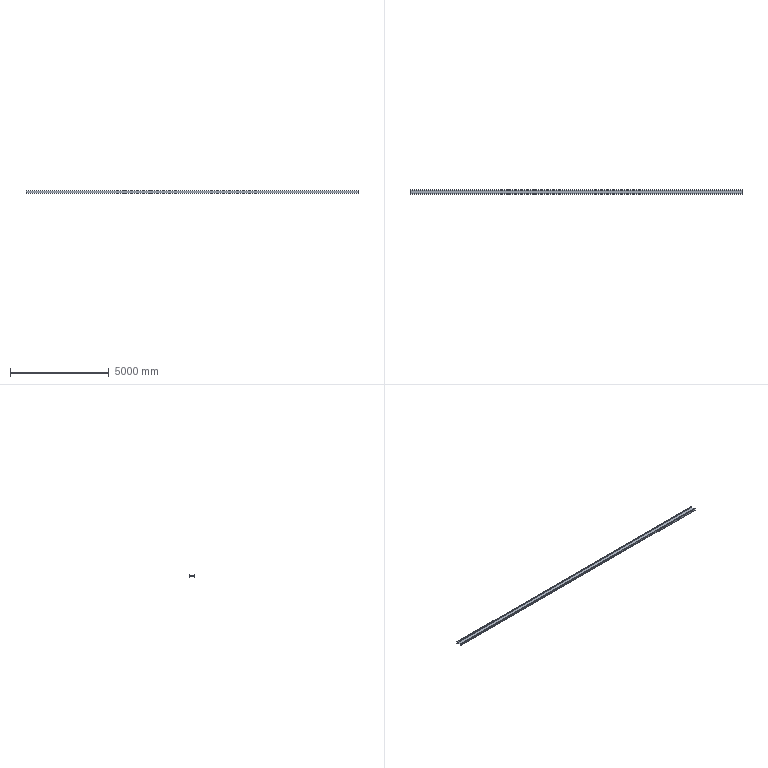Part | SolidWorks | features Fillet 2, Extrusion 1 | 1 solid | 22 faces | box 16840 x 250 x 118 mm | volume 87084540 mm3 | plane 14 | cylinder 8 | commonest cylinder face diameters 10 x4 20 x4
STEP:
#1=CARTESIAN_POINT('',(16840.,3.431,59.));
#2=VERTEX_POINT('',#1);
#3=CARTESIAN_POINT('',(16840.,0.,59.));
#4=VERTEX_POINT('',#3);
#5=CARTESIAN_POINT('',(16840.,7.667,59.));
#6=DIRECTION('',(0.,-1.,0.));
#7=VECTOR('',#6,1000.);
#8=LINE('',#5,#7);
#9=EDGE_CURVE('',#2,#4,#8,.T.);
#10=ORIENTED_EDGE('',*,*,#9,.F.);
#11=CARTESIAN_POINT('',(0.,3.431,59.));
#12=VERTEX_POINT('',#11);
#13=CARTESIAN_POINT('',(16840.,3.431,59.));
#14=DIRECTION('',(-1.,0.,0.));
#15=VECTOR('',#14,1000.);
#16=LINE('',#13,#15);
#17=EDGE_CURVE('',#2,#12,#16,.T.);
#18=ORIENTED_EDGE('',*,*,#17,.T.);
#19=CARTESIAN_POINT('',(0.,0.,59.));
#20=VERTEX_POINT('',#19);
#21=CARTESIAN_POINT('',(0.,7.667,59.));
#22=DIRECTION('',(0.,-1.,0.));
#23=VECTOR('',#22,1000.);
#24=LINE('',#21,#23);
#25=EDGE_CURVE('',#12,#20,#24,.T.);
#26=ORIENTED_EDGE('',*,*,#25,.T.);
#27=CARTESIAN_POINT('',(16840.,0.,59.));
#28=DIRECTION('',(-1.,0.,0.));
#29=VECTOR('',#28,1000.);
#30=LINE('',#27,#29);
#31=EDGE_CURVE('',#4,#20,#30,.T.);
#32=ORIENTED_EDGE('',*,*,#31,.F.);
#33=EDGE_LOOP('',(#10,#18,#26,#32));
#34=FACE_OUTER_BOUND('',#33,.T.);
#35=CARTESIAN_POINT('',(16840.,7.667,59.));
#36=DIRECTION('',(0.,0.,-1.));
#37=DIRECTION('',(-1.,0.,0.));
#38=AXIS2_PLACEMENT_3D('',#35,#36,#37);
#39=PLANE('',#38);
#40=ADVANCED_FACE('',(#34),#39,.F.);
#41=CARTESIAN_POINT('',(0.,0.,-59.));
#42=VERTEX_POINT('',#41);
#43=CARTESIAN_POINT('',(0.,0.,59.));
#44=DIRECTION('',(0.,0.,-1.));
#45=VECTOR('',#44,1000.);
#46=LINE('',#43,#45);
#47=EDGE_CURVE('',#20,#42,#46,.T.);
#48=ORIENTED_EDGE('',*,*,#47,.T.);
#49=CARTESIAN_POINT('',(16840.,0.,-59.));
#50=VERTEX_POINT('',#49);
#51=CARTESIAN_POINT('',(16840.,0.,-59.));
#52=DIRECTION('',(-1.,0.,0.));
#53=VECTOR('',#52,1000.);
#54=LINE('',#51,#53);
#55=EDGE_CURVE('',#50,#42,#54,.T.);
#56=ORIENTED_EDGE('',*,*,#55,.F.);
#57=CARTESIAN_POINT('',(16840.,0.,59.));
#58=DIRECTION('',(0.,0.,-1.));
#59=VECTOR('',#58,1000.);
#60=LINE('',#57,#59);
#61=EDGE_CURVE('',#4,#50,#60,.T.);
#62=ORIENTED_EDGE('',*,*,#61,.F.);
#63=ORIENTED_EDGE('',*,*,#31,.T.);
#64=EDGE_LOOP('',(#48,#56,#62,#63));
#65=FACE_OUTER_BOUND('',#64,.T.);
#66=CARTESIAN_POINT('',(16840.,0.,59.));
#67=DIRECTION('',(0.,1.,0.));
#68=DIRECTION('',(0.,0.,1.));
#69=AXIS2_PLACEMENT_3D('',#66,#67,#68);
#70=PLANE('',#69);
#71=ADVANCED_FACE('',(#65),#70,.F.);
#72=CARTESIAN_POINT('',(0.,3.431,-59.));
#73=VERTEX_POINT('',#72);
#74=CARTESIAN_POINT('',(0.,7.667,-59.));
#75=DIRECTION('',(0.,1.,0.));
#76=VECTOR('',#75,1000.);
#77=LINE('',#74,#76);
#78=EDGE_CURVE('',#42,#73,#77,.T.);
#79=ORIENTED_EDGE('',*,*,#78,.T.);
#80=CARTESIAN_POINT('',(16840.,3.431,-59.));
#81=VERTEX_POINT('',#80);
#82=CARTESIAN_POINT('',(16840.,3.431,-59.));
#83=DIRECTION('',(1.,0.,0.));
#84=VECTOR('',#83,1000.);
#85=LINE('',#82,#84);
#86=EDGE_CURVE('',#73,#81,#85,.T.);
#87=ORIENTED_EDGE('',*,*,#86,.T.);
#88=CARTESIAN_POINT('',(16840.,7.667,-59.));
#89=DIRECTION('',(0.,1.,0.));
#90=VECTOR('',#89,1000.);
#91=LINE('',#88,#90);
#92=EDGE_CURVE('',#50,#81,#91,.T.);
#93=ORIENTED_EDGE('',*,*,#92,.F.);
#94=ORIENTED_EDGE('',*,*,#55,.T.);
#95=EDGE_LOOP('',(#79,#87,#93,#94));
#96=FACE_OUTER_BOUND('',#95,.T.);
#97=CARTESIAN_POINT('',(16840.,7.667,-59.));
#98=DIRECTION('',(0.,0.,1.));
#99=DIRECTION('',(1.,0.,0.));
#100=AXIS2_PLACEMENT_3D('',#97,#98,#99);
#101=PLANE('',#100);
#102=ADVANCED_FACE('',(#96),#101,.F.);
#103=CARTESIAN_POINT('',(16840.,8.363,-54.822));
#104=VERTEX_POINT('',#103);
#105=CARTESIAN_POINT('',(16840.,15.274,-13.356));
#106=VERTEX_POINT('',#105);
#107=CARTESIAN_POINT('',(16840.,16.667,-5.));
#108=DIRECTION('',(0.,0.1644,0.9864));
#109=VECTOR('',#108,1000.);
#110=LINE('',#107,#109);
#111=EDGE_CURVE('',#104,#106,#110,.T.);
#112=ORIENTED_EDGE('',*,*,#111,.F.);
#113=CARTESIAN_POINT('',(0.,8.363,-54.822));
#114=VERTEX_POINT('',#113);
#115=CARTESIAN_POINT('',(16840.,8.363,-54.822));
#116=DIRECTION('',(-1.,0.,0.));
#117=VECTOR('',#116,1000.);
#118=LINE('',#115,#117);
#119=EDGE_CURVE('',#104,#114,#118,.T.);
#120=ORIENTED_EDGE('',*,*,#119,.T.);
#121=CARTESIAN_POINT('',(0.,15.274,-13.356));
#122=VERTEX_POINT('',#121);
#123=CARTESIAN_POINT('',(0.,16.667,-5.));
#124=DIRECTION('',(0.,0.1644,0.9864));
#125=VECTOR('',#124,1000.);
#126=LINE('',#123,#125);
#127=EDGE_CURVE('',#114,#122,#126,.T.);
#128=ORIENTED_EDGE('',*,*,#127,.T.);
#129=CARTESIAN_POINT('',(16840.,15.274,-13.356));
#130=DIRECTION('',(1.,0.,0.));
#131=VECTOR('',#130,1000.);
#132=LINE('',#129,#131);
#133=EDGE_CURVE('',#122,#106,#132,.T.);
#134=ORIENTED_EDGE('',*,*,#133,.T.);
#135=EDGE_LOOP('',(#112,#120,#128,#134));
#136=FACE_OUTER_BOUND('',#135,.T.);
#137=CARTESIAN_POINT('',(16840.,16.667,-5.));
#138=DIRECTION('',(0.,-0.9864,0.1644));
#139=DIRECTION('',(0.,-0.1644,-0.9864));
#140=AXIS2_PLACEMENT_3D('',#137,#138,#139);
#141=PLANE('',#140);
#142=ADVANCED_FACE('',(#136),#141,.F.);
#143=CARTESIAN_POINT('',(0.,25.138,-5.));
#144=VERTEX_POINT('',#143);
#145=CARTESIAN_POINT('',(0.,224.862,-5.));
#146=VERTEX_POINT('',#145);
#147=CARTESIAN_POINT('',(0.,233.333,-5.));
#148=DIRECTION('',(0.,1.,0.));
#149=VECTOR('',#148,1000.);
#150=LINE('',#147,#149);
#151=EDGE_CURVE('',#144,#146,#150,.T.);
#152=ORIENTED_EDGE('',*,*,#151,.T.);
#153=CARTESIAN_POINT('',(16840.,224.862,-5.));
#154=VERTEX_POINT('',#153);
#155=CARTESIAN_POINT('',(16840.,224.862,-5.));
#156=DIRECTION('',(1.,0.,0.));
#157=VECTOR('',#156,1000.);
#158=LINE('',#155,#157);
#159=EDGE_CURVE('',#146,#154,#158,.T.);
#160=ORIENTED_EDGE('',*,*,#159,.T.);
#161=CARTESIAN_POINT('',(16840.,25.138,-5.));
#162=VERTEX_POINT('',#161);
#163=CARTESIAN_POINT('',(16840.,233.333,-5.));
#164=DIRECTION('',(0.,1.,0.));
#165=VECTOR('',#164,1000.);
#166=LINE('',#163,#165);
#167=EDGE_CURVE('',#162,#154,#166,.T.);
#168=ORIENTED_EDGE('',*,*,#167,.F.);
#169=CARTESIAN_POINT('',(0.,25.138,-5.));
#170=DIRECTION('',(-1.,0.,0.));
#171=VECTOR('',#170,1000.);
#172=LINE('',#169,#171);
#173=EDGE_CURVE('',#162,#144,#172,.T.);
#174=ORIENTED_EDGE('',*,*,#173,.T.);
#175=EDGE_LOOP('',(#152,#160,#168,#174));
#176=FACE_OUTER_BOUND('',#175,.T.);
#177=CARTESIAN_POINT('',(16840.,233.333,-5.));
#178=DIRECTION('',(0.,0.,1.));
#179=DIRECTION('',(0.,-1.,0.));
#180=AXIS2_PLACEMENT_3D('',#177,#178,#179);
#181=PLANE('',#180);
#182=ADVANCED_FACE('',(#176),#181,.F.);
#183=CARTESIAN_POINT('',(0.,234.726,-13.356));
#184=VERTEX_POINT('',#183);
#185=CARTESIAN_POINT('',(0.,241.637,-54.822));
#186=VERTEX_POINT('',#185);
#187=CARTESIAN_POINT('',(0.,242.333,-59.));
#188=DIRECTION('',(0.,0.1644,-0.9864));
#189=VECTOR('',#188,1000.);
#190=LINE('',#187,#189);
#191=EDGE_CURVE('',#184,#186,#190,.T.);
#192=ORIENTED_EDGE('',*,*,#191,.T.);
#193=CARTESIAN_POINT('',(16840.,241.637,-54.822));
#194=VERTEX_POINT('',#193);
#195=CARTESIAN_POINT('',(16840.,241.637,-54.822));
#196=DIRECTION('',(1.,0.,0.));
#197=VECTOR('',#196,1000.);
#198=LINE('',#195,#197);
#199=EDGE_CURVE('',#186,#194,#198,.T.);
#200=ORIENTED_EDGE('',*,*,#199,.T.);
#201=CARTESIAN_POINT('',(16840.,234.726,-13.356));
#202=VERTEX_POINT('',#201);
#203=CARTESIAN_POINT('',(16840.,242.333,-59.));
#204=DIRECTION('',(0.,0.1644,-0.9864));
#205=VECTOR('',#204,1000.);
#206=LINE('',#203,#205);
#207=EDGE_CURVE('',#202,#194,#206,.T.);
#208=ORIENTED_EDGE('',*,*,#207,.F.);
#209=CARTESIAN_POINT('',(0.,234.726,-13.356));
#210=DIRECTION('',(-1.,0.,0.));
#211=VECTOR('',#210,1000.);
#212=LINE('',#209,#211);
#213=EDGE_CURVE('',#202,#184,#212,.T.);
#214=ORIENTED_EDGE('',*,*,#213,.T.);
#215=EDGE_LOOP('',(#192,#200,#208,#214));
#216=FACE_OUTER_BOUND('',#215,.T.);
#217=CARTESIAN_POINT('',(16840.,242.333,-59.));
#218=DIRECTION('',(0.,0.9864,0.1644));
#219=DIRECTION('',(0.,-0.1644,0.9864));
#220=AXIS2_PLACEMENT_3D('',#217,#218,#219);
#221=PLANE('',#220);
#222=ADVANCED_FACE('',(#216),#221,.F.);
#223=CARTESIAN_POINT('',(16840.,246.569,-59.));
#224=VERTEX_POINT('',#223);
#225=CARTESIAN_POINT('',(16840.,250.,-59.));
#226=VERTEX_POINT('',#225);
#227=CARTESIAN_POINT('',(16840.,250.,-59.));
#228=DIRECTION('',(0.,1.,0.));
#229=VECTOR('',#228,1000.);
#230=LINE('',#227,#229);
#231=EDGE_CURVE('',#224,#226,#230,.T.);
#232=ORIENTED_EDGE('',*,*,#231,.F.);
#233=CARTESIAN_POINT('',(0.,246.569,-59.));
#234=VERTEX_POINT('',#233);
#235=CARTESIAN_POINT('',(16840.,246.569,-59.));
#236=DIRECTION('',(-1.,0.,0.));
#237=VECTOR('',#236,1000.);
#238=LINE('',#235,#237);
#239=EDGE_CURVE('',#224,#234,#238,.T.);
#240=ORIENTED_EDGE('',*,*,#239,.T.);
#241=CARTESIAN_POINT('',(0.,250.,-59.));
#242=VERTEX_POINT('',#241);
#243=CARTESIAN_POINT('',(0.,250.,-59.));
#244=DIRECTION('',(0.,1.,0.));
#245=VECTOR('',#244,1000.);
#246=LINE('',#243,#245);
#247=EDGE_CURVE('',#234,#242,#246,.T.);
#248=ORIENTED_EDGE('',*,*,#247,.T.);
#249=CARTESIAN_POINT('',(16840.,250.,-59.));
#250=DIRECTION('',(-1.,0.,0.));
#251=VECTOR('',#250,1000.);
#252=LINE('',#249,#251);
#253=EDGE_CURVE('',#226,#242,#252,.T.);
#254=ORIENTED_EDGE('',*,*,#253,.F.);
#255=EDGE_LOOP('',(#232,#240,#248,#254));
#256=FACE_OUTER_BOUND('',#255,.T.);
#257=CARTESIAN_POINT('',(16840.,250.,-59.));
#258=DIRECTION('',(0.,0.,1.));
#259=DIRECTION('',(0.,-1.,0.));
#260=AXIS2_PLACEMENT_3D('',#257,#258,#259);
#261=PLANE('',#260);
#262=ADVANCED_FACE('',(#256),#261,.F.);
#263=CARTESIAN_POINT('',(0.,250.,59.));
#264=VERTEX_POINT('',#263);
#265=CARTESIAN_POINT('',(0.,250.,59.));
#266=DIRECTION('',(0.,0.,1.));
#267=VECTOR('',#266,1000.);
#268=LINE('',#265,#267);
#269=EDGE_CURVE('',#242,#264,#268,.T.);
#270=ORIENTED_EDGE('',*,*,#269,.T.);
#271=CARTESIAN_POINT('',(16840.,250.,59.));
#272=VERTEX_POINT('',#271);
#273=CARTESIAN_POINT('',(16840.,250.,59.));
#274=DIRECTION('',(-1.,0.,0.));
#275=VECTOR('',#274,1000.);
#276=LINE('',#273,#275);
#277=EDGE_CURVE('',#272,#264,#276,.T.);
#278=ORIENTED_EDGE('',*,*,#277,.F.);
#279=CARTESIAN_POINT('',(16840.,250.,59.));
#280=DIRECTION('',(0.,0.,1.));
#281=VECTOR('',#280,1000.);
#282=LINE('',#279,#281);
#283=EDGE_CURVE('',#226,#272,#282,.T.);
#284=ORIENTED_EDGE('',*,*,#283,.F.);
#285=ORIENTED_EDGE('',*,*,#253,.T.);
#286=EDGE_LOOP('',(#270,#278,#284,#285));
#287=FACE_OUTER_BOUND('',#286,.T.);
#288=CARTESIAN_POINT('',(16840.,250.,59.));
#289=DIRECTION('',(0.,-1.,0.));
#290=DIRECTION('',(0.,0.,-1.));
#291=AXIS2_PLACEMENT_3D('',#288,#289,#290);
#292=PLANE('',#291);
#293=ADVANCED_FACE('',(#287),#292,.F.);
#294=CARTESIAN_POINT('',(0.,246.569,59.));
#295=VERTEX_POINT('',#294);
#296=CARTESIAN_POINT('',(0.,250.,59.));
#297=DIRECTION('',(0.,-1.,0.));
#298=VECTOR('',#297,1000.);
#299=LINE('',#296,#298);
#300=EDGE_CURVE('',#264,#295,#299,.T.);
#301=ORIENTED_EDGE('',*,*,#300,.T.);
#302=CARTESIAN_POINT('',(16840.,246.569,59.));
#303=VERTEX_POINT('',#302);
#304=CARTESIAN_POINT('',(16840.,246.569,59.));
#305=DIRECTION('',(1.,0.,0.));
#306=VECTOR('',#305,1000.);
#307=LINE('',#304,#306);
#308=EDGE_CURVE('',#295,#303,#307,.T.);
#309=ORIENTED_EDGE('',*,*,#308,.T.);
#310=CARTESIAN_POINT('',(16840.,250.,59.));
#311=DIRECTION('',(0.,-1.,0.));
#312=VECTOR('',#311,1000.);
#313=LINE('',#310,#312);
#314=EDGE_CURVE('',#272,#303,#313,.T.);
#315=ORIENTED_EDGE('',*,*,#314,.F.);
#316=ORIENTED_EDGE('',*,*,#277,.T.);
#317=EDGE_LOOP('',(#301,#309,#315,#316));
#318=FACE_OUTER_BOUND('',#317,.T.);
#319=CARTESIAN_POINT('',(16840.,250.,59.));
#320=DIRECTION('',(0.,0.,-1.));
#321=DIRECTION('',(-1.,0.,0.));
#322=AXIS2_PLACEMENT_3D('',#319,#320,#321);
#323=PLANE('',#322);
#324=ADVANCED_FACE('',(#318),#323,.F.);
#325=CARTESIAN_POINT('',(16840.,241.637,54.822));
#326=VERTEX_POINT('',#325);
#327=CARTESIAN_POINT('',(16840.,234.726,13.356));
#328=VERTEX_POINT('',#327);
#329=CARTESIAN_POINT('',(16840.,242.333,59.));
#330=DIRECTION('',(0.,-0.1644,-0.9864));
#331=VECTOR('',#330,1000.);
#332=LINE('',#329,#331);
#333=EDGE_CURVE('',#326,#328,#332,.T.);
#334=ORIENTED_EDGE('',*,*,#333,.F.);
#335=CARTESIAN_POINT('',(0.,241.637,54.822));
#336=VERTEX_POINT('',#335);
#337=CARTESIAN_POINT('',(16840.,241.637,54.822));
#338=DIRECTION('',(-1.,0.,0.));
#339=VECTOR('',#338,1000.);
#340=LINE('',#337,#339);
#341=EDGE_CURVE('',#326,#336,#340,.T.);
#342=ORIENTED_EDGE('',*,*,#341,.T.);
#343=CARTESIAN_POINT('',(0.,234.726,13.356));
#344=VERTEX_POINT('',#343);
#345=CARTESIAN_POINT('',(0.,242.333,59.));
#346=DIRECTION('',(0.,-0.1644,-0.9864));
#347=VECTOR('',#346,1000.);
#348=LINE('',#345,#347);
#349=EDGE_CURVE('',#336,#344,#348,.T.);
#350=ORIENTED_EDGE('',*,*,#349,.T.);
#351=CARTESIAN_POINT('',(16840.,234.726,13.356));
#352=DIRECTION('',(1.,0.,0.));
#353=VECTOR('',#352,1000.);
#354=LINE('',#351,#353);
#355=EDGE_CURVE('',#344,#328,#354,.T.);
#356=ORIENTED_EDGE('',*,*,#355,.T.);
#357=EDGE_LOOP('',(#334,#342,#350,#356));
#358=FACE_OUTER_BOUND('',#357,.T.);
#359=CARTESIAN_POINT('',(16840.,242.333,59.));
#360=DIRECTION('',(0.,0.9864,-0.1644));
#361=DIRECTION('',(0.,0.1644,0.9864));
#362=AXIS2_PLACEMENT_3D('',#359,#360,#361);
#363=PLANE('',#362);
#364=ADVANCED_FACE('',(#358),#363,.F.);
#365=CARTESIAN_POINT('',(0.,224.862,5.));
#366=VERTEX_POINT('',#365);
#367=CARTESIAN_POINT('',(0.,25.138,5.));
#368=VERTEX_POINT('',#367);
#369=CARTESIAN_POINT('',(0.,233.333,5.));
#370=DIRECTION('',(0.,-1.,0.));
#371=VECTOR('',#370,1000.);
#372=LINE('',#369,#371);
#373=EDGE_CURVE('',#366,#368,#372,.T.);
#374=ORIENTED_EDGE('',*,*,#373,.T.);
#375=CARTESIAN_POINT('',(16840.,25.138,5.));
#376=VERTEX_POINT('',#375);
#377=CARTESIAN_POINT('',(16840.,25.138,5.));
#378=DIRECTION('',(1.,0.,0.));
#379=VECTOR('',#378,1000.);
#380=LINE('',#377,#379);
#381=EDGE_CURVE('',#368,#376,#380,.T.);
#382=ORIENTED_EDGE('',*,*,#381,.T.);
#383=CARTESIAN_POINT('',(16840.,224.862,5.));
#384=VERTEX_POINT('',#383);
#385=CARTESIAN_POINT('',(16840.,233.333,5.));
#386=DIRECTION('',(0.,-1.,0.));
#387=VECTOR('',#386,1000.);
#388=LINE('',#385,#387);
#389=EDGE_CURVE('',#384,#376,#388,.T.);
#390=ORIENTED_EDGE('',*,*,#389,.F.);
#391=CARTESIAN_POINT('',(0.,224.862,5.));
#392=DIRECTION('',(-1.,0.,0.));
#393=VECTOR('',#392,1000.);
#394=LINE('',#391,#393);
#395=EDGE_CURVE('',#384,#366,#394,.T.);
#396=ORIENTED_EDGE('',*,*,#395,.T.);
#397=EDGE_LOOP('',(#374,#382,#390,#396));
#398=FACE_OUTER_BOUND('',#397,.T.);
#399=CARTESIAN_POINT('',(16840.,233.333,5.));
#400=DIRECTION('',(0.,0.,-1.));
#401=DIRECTION('',(0.,1.,0.));
#402=AXIS2_PLACEMENT_3D('',#399,#400,#401);
#403=PLANE('',#402);
#404=ADVANCED_FACE('',(#398),#403,.F.);
#405=CARTESIAN_POINT('',(0.,15.274,13.356));
#406=VERTEX_POINT('',#405);
#407=CARTESIAN_POINT('',(0.,8.363,54.822));
#408=VERTEX_POINT('',#407);
#409=CARTESIAN_POINT('',(0.,16.667,5.));
#410=DIRECTION('',(0.,-0.1644,0.9864));
#411=VECTOR('',#410,1000.);
#412=LINE('',#409,#411);
#413=EDGE_CURVE('',#406,#408,#412,.T.);
#414=ORIENTED_EDGE('',*,*,#413,.T.);
#415=CARTESIAN_POINT('',(16840.,8.363,54.822));
#416=VERTEX_POINT('',#415);
#417=CARTESIAN_POINT('',(16840.,8.363,54.822));
#418=DIRECTION('',(1.,0.,0.));
#419=VECTOR('',#418,1000.);
#420=LINE('',#417,#419);
#421=EDGE_CURVE('',#408,#416,#420,.T.);
#422=ORIENTED_EDGE('',*,*,#421,.T.);
#423=CARTESIAN_POINT('',(16840.,15.274,13.356));
#424=VERTEX_POINT('',#423);
#425=CARTESIAN_POINT('',(16840.,16.667,5.));
#426=DIRECTION('',(0.,-0.1644,0.9864));
#427=VECTOR('',#426,1000.);
#428=LINE('',#425,#427);
#429=EDGE_CURVE('',#424,#416,#428,.T.);
#430=ORIENTED_EDGE('',*,*,#429,.F.);
#431=CARTESIAN_POINT('',(0.,15.274,13.356));
#432=DIRECTION('',(-1.,0.,0.));
#433=VECTOR('',#432,1000.);
#434=LINE('',#431,#433);
#435=EDGE_CURVE('',#424,#406,#434,.T.);
#436=ORIENTED_EDGE('',*,*,#435,.T.);
#437=EDGE_LOOP('',(#414,#422,#430,#436));
#438=FACE_OUTER_BOUND('',#437,.T.);
#439=CARTESIAN_POINT('',(16840.,16.667,5.));
#440=DIRECTION('',(0.,-0.9864,-0.1644));
#441=DIRECTION('',(0.,0.1644,-0.9864));
#442=AXIS2_PLACEMENT_3D('',#439,#440,#441);
#443=PLANE('',#442);
#444=ADVANCED_FACE('',(#438),#443,.F.);
#445=ORIENTED_EDGE('',*,*,#314,.T.);
#446=CARTESIAN_POINT('',(16840.,246.569,54.));
#447=DIRECTION('',(1.,0.,0.));
#448=DIRECTION('',(0.,0.,-1.));
#449=AXIS2_PLACEMENT_3D('',#446,#447,#448);
#450=CIRCLE('',#449,5.);
#451=EDGE_CURVE('',#303,#326,#450,.T.);
#452=ORIENTED_EDGE('',*,*,#451,.T.);
#453=ORIENTED_EDGE('',*,*,#333,.T.);
#454=CARTESIAN_POINT('',(16840.,224.862,15.));
#455=DIRECTION('',(-1.,0.,0.));
#456=DIRECTION('',(0.,0.,-1.));
#457=AXIS2_PLACEMENT_3D('',#454,#455,#456);
#458=CIRCLE('',#457,10.);
#459=EDGE_CURVE('',#328,#384,#458,.T.);
#460=ORIENTED_EDGE('',*,*,#459,.T.);
#461=ORIENTED_EDGE('',*,*,#389,.T.);
#462=CARTESIAN_POINT('',(16840.,25.138,15.));
#463=DIRECTION('',(-1.,0.,0.));
#464=DIRECTION('',(0.,0.,-1.));
#465=AXIS2_PLACEMENT_3D('',#462,#463,#464);
#466=CIRCLE('',#465,10.);
#467=EDGE_CURVE('',#376,#424,#466,.T.);
#468=ORIENTED_EDGE('',*,*,#467,.T.);
#469=ORIENTED_EDGE('',*,*,#429,.T.);
#470=CARTESIAN_POINT('',(16840.,3.431,54.));
#471=DIRECTION('',(1.,0.,0.));
#472=DIRECTION('',(0.,0.,-1.));
#473=AXIS2_PLACEMENT_3D('',#470,#471,#472);
#474=CIRCLE('',#473,5.);
#475=EDGE_CURVE('',#416,#2,#474,.T.);
#476=ORIENTED_EDGE('',*,*,#475,.T.);
#477=ORIENTED_EDGE('',*,*,#9,.T.);
#478=ORIENTED_EDGE('',*,*,#61,.T.);
#479=ORIENTED_EDGE('',*,*,#92,.T.);
#480=CARTESIAN_POINT('',(16840.,3.431,-54.));
#481=DIRECTION('',(1.,0.,0.));
#482=DIRECTION('',(0.,0.,-1.));
#483=AXIS2_PLACEMENT_3D('',#480,#481,#482);
#484=CIRCLE('',#483,5.);
#485=EDGE_CURVE('',#81,#104,#484,.T.);
#486=ORIENTED_EDGE('',*,*,#485,.T.);
#487=ORIENTED_EDGE('',*,*,#111,.T.);
#488=CARTESIAN_POINT('',(16840.,25.138,-15.));
#489=DIRECTION('',(-1.,0.,0.));
#490=DIRECTION('',(0.,0.,-1.));
#491=AXIS2_PLACEMENT_3D('',#488,#489,#490);
#492=CIRCLE('',#491,10.);
#493=EDGE_CURVE('',#106,#162,#492,.T.);
#494=ORIENTED_EDGE('',*,*,#493,.T.);
#495=ORIENTED_EDGE('',*,*,#167,.T.);
#496=CARTESIAN_POINT('',(16840.,224.862,-15.));
#497=DIRECTION('',(-1.,0.,0.));
#498=DIRECTION('',(0.,0.,-1.));
#499=AXIS2_PLACEMENT_3D('',#496,#497,#498);
#500=CIRCLE('',#499,10.);
#501=EDGE_CURVE('',#154,#202,#500,.T.);
#502=ORIENTED_EDGE('',*,*,#501,.T.);
#503=ORIENTED_EDGE('',*,*,#207,.T.);
#504=CARTESIAN_POINT('',(16840.,246.569,-54.));
#505=DIRECTION('',(1.,0.,0.));
#506=DIRECTION('',(0.,0.,-1.));
#507=AXIS2_PLACEMENT_3D('',#504,#505,#506);
#508=CIRCLE('',#507,5.);
#509=EDGE_CURVE('',#194,#224,#508,.T.);
#510=ORIENTED_EDGE('',*,*,#509,.T.);
#511=ORIENTED_EDGE('',*,*,#231,.T.);
#512=ORIENTED_EDGE('',*,*,#283,.T.);
#513=EDGE_LOOP('',(#445,#452,#453,#460,#461,#468,#469,#476,#477,#478,#479,#486,#487,#494,#495,#502,#503,#510,#511,#512));
#514=FACE_OUTER_BOUND('',#513,.T.);
#515=CARTESIAN_POINT('',(16840.,250.,59.));
#516=DIRECTION('',(1.,0.,0.));
#517=DIRECTION('',(0.,0.,-1.));
#518=AXIS2_PLACEMENT_3D('',#515,#516,#517);
#519=PLANE('',#518);
#520=ADVANCED_FACE('',(#514),#519,.T.);
#521=ORIENTED_EDGE('',*,*,#349,.F.);
#522=CARTESIAN_POINT('',(0.,246.569,54.));
#523=DIRECTION('',(-1.,0.,0.));
#524=DIRECTION('',(0.,0.,-1.));
#525=AXIS2_PLACEMENT_3D('',#522,#523,#524);
#526=CIRCLE('',#525,5.);
#527=EDGE_CURVE('',#336,#295,#526,.T.);
#528=ORIENTED_EDGE('',*,*,#527,.T.);
#529=ORIENTED_EDGE('',*,*,#300,.F.);
#530=ORIENTED_EDGE('',*,*,#269,.F.);
#531=ORIENTED_EDGE('',*,*,#247,.F.);
#532=CARTESIAN_POINT('',(0.,246.569,-54.));
#533=DIRECTION('',(-1.,0.,0.));
#534=DIRECTION('',(0.,0.,-1.));
#535=AXIS2_PLACEMENT_3D('',#532,#533,#534);
#536=CIRCLE('',#535,5.);
#537=EDGE_CURVE('',#234,#186,#536,.T.);
#538=ORIENTED_EDGE('',*,*,#537,.T.);
#539=ORIENTED_EDGE('',*,*,#191,.F.);
#540=CARTESIAN_POINT('',(0.,224.862,-15.));
#541=DIRECTION('',(1.,0.,0.));
#542=DIRECTION('',(0.,0.,-1.));
#543=AXIS2_PLACEMENT_3D('',#540,#541,#542);
#544=CIRCLE('',#543,10.);
#545=EDGE_CURVE('',#184,#146,#544,.T.);
#546=ORIENTED_EDGE('',*,*,#545,.T.);
#547=ORIENTED_EDGE('',*,*,#151,.F.);
#548=CARTESIAN_POINT('',(0.,25.138,-15.));
#549=DIRECTION('',(1.,0.,0.));
#550=DIRECTION('',(0.,0.,-1.));
#551=AXIS2_PLACEMENT_3D('',#548,#549,#550);
#552=CIRCLE('',#551,10.);
#553=EDGE_CURVE('',#144,#122,#552,.T.);
#554=ORIENTED_EDGE('',*,*,#553,.T.);
#555=ORIENTED_EDGE('',*,*,#127,.F.);
#556=CARTESIAN_POINT('',(0.,3.431,-54.));
#557=DIRECTION('',(-1.,0.,0.));
#558=DIRECTION('',(0.,0.,-1.));
#559=AXIS2_PLACEMENT_3D('',#556,#557,#558);
#560=CIRCLE('',#559,5.);
#561=EDGE_CURVE('',#114,#73,#560,.T.);
#562=ORIENTED_EDGE('',*,*,#561,.T.);
#563=ORIENTED_EDGE('',*,*,#78,.F.);
#564=ORIENTED_EDGE('',*,*,#47,.F.);
#565=ORIENTED_EDGE('',*,*,#25,.F.);
#566=CARTESIAN_POINT('',(0.,3.431,54.));
#567=DIRECTION('',(-1.,0.,0.));
#568=DIRECTION('',(0.,0.,-1.));
#569=AXIS2_PLACEMENT_3D('',#566,#567,#568);
#570=CIRCLE('',#569,5.);
#571=EDGE_CURVE('',#12,#408,#570,.T.);
#572=ORIENTED_EDGE('',*,*,#571,.T.);
#573=ORIENTED_EDGE('',*,*,#413,.F.);
#574=CARTESIAN_POINT('',(0.,25.138,15.));
#575=DIRECTION('',(1.,0.,0.));
#576=DIRECTION('',(0.,0.,-1.));
#577=AXIS2_PLACEMENT_3D('',#574,#575,#576);
#578=CIRCLE('',#577,10.);
#579=EDGE_CURVE('',#406,#368,#578,.T.);
#580=ORIENTED_EDGE('',*,*,#579,.T.);
#581=ORIENTED_EDGE('',*,*,#373,.F.);
#582=CARTESIAN_POINT('',(0.,224.862,15.));
#583=DIRECTION('',(1.,0.,0.));
#584=DIRECTION('',(0.,0.,-1.));
#585=AXIS2_PLACEMENT_3D('',#582,#583,#584);
#586=CIRCLE('',#585,10.);
#587=EDGE_CURVE('',#366,#344,#586,.T.);
#588=ORIENTED_EDGE('',*,*,#587,.T.);
#589=EDGE_LOOP('',(#521,#528,#529,#530,#531,#538,#539,#546,#547,#554,#555,#562,#563,#564,#565,#572,#573,#580,#581,#588));
#590=FACE_OUTER_BOUND('',#589,.T.);
#591=CARTESIAN_POINT('',(0.,250.,59.));
#592=DIRECTION('',(1.,0.,0.));
#593=DIRECTION('',(0.,0.,-1.));
#594=AXIS2_PLACEMENT_3D('',#591,#592,#593);
#595=PLANE('',#594);
#596=ADVANCED_FACE('',(#590),#595,.F.);
#597=ORIENTED_EDGE('',*,*,#501,.F.);
#598=ORIENTED_EDGE('',*,*,#159,.F.);
#599=ORIENTED_EDGE('',*,*,#545,.F.);
#600=ORIENTED_EDGE('',*,*,#213,.F.);
#601=EDGE_LOOP('',(#597,#598,#599,#600));
#602=FACE_OUTER_BOUND('',#601,.T.);
#603=CARTESIAN_POINT('',(16840.,224.862,-15.));
#604=DIRECTION('',(1.,0.,0.));
#605=DIRECTION('',(0.,0.,-1.));
#606=AXIS2_PLACEMENT_3D('',#603,#604,#605);
#607=CYLINDRICAL_SURFACE('',#606,10.);
#608=ADVANCED_FACE('',(#602),#607,.F.);
#609=ORIENTED_EDGE('',*,*,#493,.F.);
#610=ORIENTED_EDGE('',*,*,#133,.F.);
#611=ORIENTED_EDGE('',*,*,#553,.F.);
#612=ORIENTED_EDGE('',*,*,#173,.F.);
#613=EDGE_LOOP('',(#609,#610,#611,#612));
#614=FACE_OUTER_BOUND('',#613,.T.);
#615=CARTESIAN_POINT('',(16840.,25.138,-15.));
#616=DIRECTION('',(1.,0.,0.));
#617=DIRECTION('',(0.,0.,-1.));
#618=AXIS2_PLACEMENT_3D('',#615,#616,#617);
#619=CYLINDRICAL_SURFACE('',#618,10.);
#620=ADVANCED_FACE('',(#614),#619,.F.);
#621=ORIENTED_EDGE('',*,*,#467,.F.);
#622=ORIENTED_EDGE('',*,*,#381,.F.);
#623=ORIENTED_EDGE('',*,*,#579,.F.);
#624=ORIENTED_EDGE('',*,*,#435,.F.);
#625=EDGE_LOOP('',(#621,#622,#623,#624));
#626=FACE_OUTER_BOUND('',#625,.T.);
#627=CARTESIAN_POINT('',(16840.,25.138,15.));
#628=DIRECTION('',(1.,0.,0.));
#629=DIRECTION('',(0.,0.,-1.));
#630=AXIS2_PLACEMENT_3D('',#627,#628,#629);
#631=CYLINDRICAL_SURFACE('',#630,10.);
#632=ADVANCED_FACE('',(#626),#631,.F.);
#633=ORIENTED_EDGE('',*,*,#459,.F.);
#634=ORIENTED_EDGE('',*,*,#355,.F.);
#635=ORIENTED_EDGE('',*,*,#587,.F.);
#636=ORIENTED_EDGE('',*,*,#395,.F.);
#637=EDGE_LOOP('',(#633,#634,#635,#636));
#638=FACE_OUTER_BOUND('',#637,.T.);
#639=CARTESIAN_POINT('',(16840.,224.862,15.));
#640=DIRECTION('',(1.,0.,0.));
#641=DIRECTION('',(0.,0.,-1.));
#642=AXIS2_PLACEMENT_3D('',#639,#640,#641);
#643=CYLINDRICAL_SURFACE('',#642,10.);
#644=ADVANCED_FACE('',(#638),#643,.F.);
#645=ORIENTED_EDGE('',*,*,#451,.F.);
#646=ORIENTED_EDGE('',*,*,#308,.F.);
#647=ORIENTED_EDGE('',*,*,#527,.F.);
#648=ORIENTED_EDGE('',*,*,#341,.F.);
#649=EDGE_LOOP('',(#645,#646,#647,#648));
#650=FACE_OUTER_BOUND('',#649,.T.);
#651=CARTESIAN_POINT('',(16840.,246.569,54.));
#652=DIRECTION('',(-1.,0.,0.));
#653=DIRECTION('',(0.,0.,1.));
#654=AXIS2_PLACEMENT_3D('',#651,#652,#653);
#655=CYLINDRICAL_SURFACE('',#654,5.);
#656=ADVANCED_FACE('',(#650),#655,.T.);
#657=ORIENTED_EDGE('',*,*,#475,.F.);
#658=ORIENTED_EDGE('',*,*,#421,.F.);
#659=ORIENTED_EDGE('',*,*,#571,.F.);
#660=ORIENTED_EDGE('',*,*,#17,.F.);
#661=EDGE_LOOP('',(#657,#658,#659,#660));
#662=FACE_OUTER_BOUND('',#661,.T.);
#663=CARTESIAN_POINT('',(16840.,3.431,54.));
#664=DIRECTION('',(-1.,0.,0.));
#665=DIRECTION('',(0.,0.,1.));
#666=AXIS2_PLACEMENT_3D('',#663,#664,#665);
#667=CYLINDRICAL_SURFACE('',#666,5.);
#668=ADVANCED_FACE('',(#662),#667,.T.);
#669=ORIENTED_EDGE('',*,*,#485,.F.);
#670=ORIENTED_EDGE('',*,*,#86,.F.);
#671=ORIENTED_EDGE('',*,*,#561,.F.);
#672=ORIENTED_EDGE('',*,*,#119,.F.);
#673=EDGE_LOOP('',(#669,#670,#671,#672));
#674=FACE_OUTER_BOUND('',#673,.T.);
#675=CARTESIAN_POINT('',(16840.,3.431,-54.));
#676=DIRECTION('',(-1.,0.,0.));
#677=DIRECTION('',(0.,0.,1.));
#678=AXIS2_PLACEMENT_3D('',#675,#676,#677);
#679=CYLINDRICAL_SURFACE('',#678,5.);
#680=ADVANCED_FACE('',(#674),#679,.T.);
#681=ORIENTED_EDGE('',*,*,#509,.F.);
#682=ORIENTED_EDGE('',*,*,#199,.F.);
#683=ORIENTED_EDGE('',*,*,#537,.F.);
#684=ORIENTED_EDGE('',*,*,#239,.F.);
#685=EDGE_LOOP('',(#681,#682,#683,#684));
#686=FACE_OUTER_BOUND('',#685,.T.);
#687=CARTESIAN_POINT('',(16840.,246.569,-54.));
#688=DIRECTION('',(-1.,0.,0.));
#689=DIRECTION('',(0.,0.,1.));
#690=AXIS2_PLACEMENT_3D('',#687,#688,#689);
#691=CYLINDRICAL_SURFACE('',#690,5.);
#692=ADVANCED_FACE('',(#686),#691,.T.);
#693=CLOSED_SHELL('',(#40,#71,#102,#142,#182,#222,#262,#293,#324,#364,#404,#444,#520,#596,#608,#620,#632,#644,#656,#668,#680,#692));
#694=MANIFOLD_SOLID_BREP('',#693);
#695=CARTESIAN_POINT('',(0.,0.,0.));
#696=DIRECTION('',(0.,0.,1.));
#697=DIRECTION('',(1.,0.,0.));
#698=AXIS2_PLACEMENT_3D('',#695,#696,#697);
#699=(LENGTH_UNIT()NAMED_UNIT(*)SI_UNIT(.MILLI.,.METRE.));
#700=UNCERTAINTY_MEASURE_WITH_UNIT(LENGTH_MEASURE(0.00001),#699,'','');
#701=(NAMED_UNIT(*)PLANE_ANGLE_UNIT()SI_UNIT($,.RADIAN.));
#702=(NAMED_UNIT(*)SI_UNIT($,.STERADIAN.)SOLID_ANGLE_UNIT());
#703=(GEOMETRIC_REPRESENTATION_CONTEXT(3)GLOBAL_UNCERTAINTY_ASSIGNED_CONTEXT((#700))GLOBAL_UNIT_ASSIGNED_CONTEXT((#699,#701,#702))REPRESENTATION_CONTEXT('',''));
#704=ADVANCED_BREP_SHAPE_REPRESENTATION('',(#694,#698),#703);